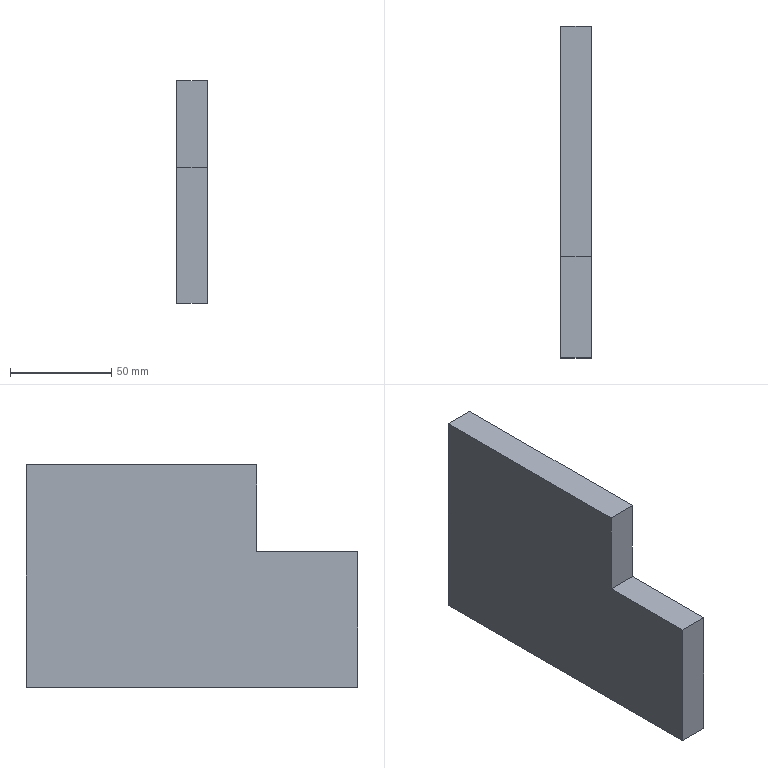Part | STEP file | Positioning_id1518_x_t | 1 solid | 8 faces | box 15 x 164 x 110 mm | volume 238350 mm3 | plane 8
STEP:
#1=CARTESIAN_POINT('',(0.,0.,0.));
#2=DIRECTION('',(0.,0.,1.));
#3=DIRECTION('',(1.,0.,0.));
#4=AXIS2_PLACEMENT_3D('',#1,#2,#3);
#5=CARTESIAN_POINT('',(-808.002,510.,100.995));
#6=VERTEX_POINT('',#5);
#7=CARTESIAN_POINT('',(-793.002,510.,100.995));
#8=VERTEX_POINT('',#7);
#9=CARTESIAN_POINT('',(-808.002,510.,100.995));
#10=DIRECTION('',(1.,0.,0.));
#11=VECTOR('',#10,1.);
#12=LINE('',#9,#11);
#13=CARTESIAN_POINT('',(-808.002,460.,100.995));
#14=DIRECTION('',(0.,0.,-1.));
#15=DIRECTION('',(-1.,0.,0.));
#16=AXIS2_PLACEMENT_3D('',#13,#14,#15);
#17=PLANE('',#16);
#18=CARTESIAN_POINT('',(0.,50.));
#19=DIRECTION('',(-1.,0.));
#20=VECTOR('',#19,1.);
#21=LINE('',#18,#20);
#22=(GEOMETRIC_REPRESENTATION_CONTEXT(2)PARAMETRIC_REPRESENTATION_CONTEXT()REPRESENTATION_CONTEXT('',''));
#23=DEFINITIONAL_REPRESENTATION('',(#21),#22);
#24=PCURVE('',#17,#23);
#25=CARTESIAN_POINT('',(-808.002,510.,133.995));
#26=DIRECTION('',(0.,-1.,0.));
#27=DIRECTION('',(-1.,0.,0.));
#28=AXIS2_PLACEMENT_3D('',#25,#26,#27);
#29=PLANE('',#28);
#30=CARTESIAN_POINT('',(0.,33.));
#31=DIRECTION('',(-1.,0.));
#32=VECTOR('',#31,1.);
#33=LINE('',#30,#32);
#34=(GEOMETRIC_REPRESENTATION_CONTEXT(2)PARAMETRIC_REPRESENTATION_CONTEXT()REPRESENTATION_CONTEXT('',''));
#35=DEFINITIONAL_REPRESENTATION('',(#33),#34);
#36=PCURVE('',#29,#35);
#37=SURFACE_CURVE('',#12,(#24,#36),.PCURVE_S1.);
#38=EDGE_CURVE('',#6,#8,#37,.T.);
#39=ORIENTED_EDGE('',*,*,#38,.F.);
#40=CARTESIAN_POINT('',(-808.002,460.,100.995));
#41=VERTEX_POINT('',#40);
#42=CARTESIAN_POINT('',(-808.002,460.,100.995));
#43=DIRECTION('',(0.,1.,0.));
#44=VECTOR('',#43,1.);
#45=LINE('',#42,#44);
#46=CARTESIAN_POINT('',(0.,0.));
#47=DIRECTION('',(0.,1.));
#48=VECTOR('',#47,1.);
#49=LINE('',#46,#48);
#50=(GEOMETRIC_REPRESENTATION_CONTEXT(2)PARAMETRIC_REPRESENTATION_CONTEXT()REPRESENTATION_CONTEXT('',''));
#51=DEFINITIONAL_REPRESENTATION('',(#49),#50);
#52=PCURVE('',#17,#51);
#53=CARTESIAN_POINT('',(-808.002,497.,63.995));
#54=DIRECTION('',(-1.,0.,0.));
#55=DIRECTION('',(0.,0.,-1.));
#56=AXIS2_PLACEMENT_3D('',#53,#54,#55);
#57=PLANE('',#56);
#58=CARTESIAN_POINT('',(-37.,37.));
#59=DIRECTION('',(0.,-1.));
#60=VECTOR('',#59,1.);
#61=LINE('',#58,#60);
#62=(GEOMETRIC_REPRESENTATION_CONTEXT(2)PARAMETRIC_REPRESENTATION_CONTEXT()REPRESENTATION_CONTEXT('',''));
#63=DEFINITIONAL_REPRESENTATION('',(#61),#62);
#64=PCURVE('',#57,#63);
#65=SURFACE_CURVE('',#45,(#52,#64),.PCURVE_S1.);
#66=EDGE_CURVE('',#41,#6,#65,.T.);
#67=ORIENTED_EDGE('',*,*,#66,.F.);
#68=CARTESIAN_POINT('',(-793.002,460.,100.995));
#69=VERTEX_POINT('',#68);
#70=CARTESIAN_POINT('',(-808.002,460.,100.995));
#71=DIRECTION('',(1.,0.,0.));
#72=VECTOR('',#71,1.);
#73=LINE('',#70,#72);
#74=CARTESIAN_POINT('',(0.,0.));
#75=DIRECTION('',(-1.,0.));
#76=VECTOR('',#75,1.);
#77=LINE('',#74,#76);
#78=(GEOMETRIC_REPRESENTATION_CONTEXT(2)PARAMETRIC_REPRESENTATION_CONTEXT()REPRESENTATION_CONTEXT('',''));
#79=DEFINITIONAL_REPRESENTATION('',(#77),#78);
#80=PCURVE('',#17,#79);
#81=CARTESIAN_POINT('',(-813.002,460.,63.995));
#82=DIRECTION('',(0.,-1.,0.));
#83=DIRECTION('',(-1.,0.,0.));
#84=AXIS2_PLACEMENT_3D('',#81,#82,#83);
#85=PLANE('',#84);
#86=CARTESIAN_POINT('',(-5.,-37.));
#87=DIRECTION('',(-1.,0.));
#88=VECTOR('',#87,1.);
#89=LINE('',#86,#88);
#90=(GEOMETRIC_REPRESENTATION_CONTEXT(2)PARAMETRIC_REPRESENTATION_CONTEXT()REPRESENTATION_CONTEXT('',''));
#91=DEFINITIONAL_REPRESENTATION('',(#89),#90);
#92=PCURVE('',#85,#91);
#93=SURFACE_CURVE('',#73,(#80,#92),.PCURVE_S1.);
#94=EDGE_CURVE('',#41,#69,#93,.T.);
#95=ORIENTED_EDGE('',*,*,#94,.T.);
#96=CARTESIAN_POINT('',(-793.002,460.,100.995));
#97=DIRECTION('',(0.,1.,0.));
#98=VECTOR('',#97,1.);
#99=LINE('',#96,#98);
#100=CARTESIAN_POINT('',(-15.,0.));
#101=DIRECTION('',(0.,1.));
#102=VECTOR('',#101,1.);
#103=LINE('',#100,#102);
#104=(GEOMETRIC_REPRESENTATION_CONTEXT(2)PARAMETRIC_REPRESENTATION_CONTEXT()REPRESENTATION_CONTEXT('',''));
#105=DEFINITIONAL_REPRESENTATION('',(#103),#104);
#106=PCURVE('',#17,#105);
#107=CARTESIAN_POINT('',(-793.002,497.,63.995));
#108=DIRECTION('',(1.,0.,0.));
#109=DIRECTION('',(0.,0.,1.));
#110=AXIS2_PLACEMENT_3D('',#107,#108,#109);
#111=PLANE('',#110);
#112=CARTESIAN_POINT('',(37.,37.));
#113=DIRECTION('',(0.,-1.));
#114=VECTOR('',#113,1.);
#115=LINE('',#112,#114);
#116=(GEOMETRIC_REPRESENTATION_CONTEXT(2)PARAMETRIC_REPRESENTATION_CONTEXT()REPRESENTATION_CONTEXT('',''));
#117=DEFINITIONAL_REPRESENTATION('',(#115),#116);
#118=PCURVE('',#111,#117);
#119=SURFACE_CURVE('',#99,(#106,#118),.PCURVE_S1.);
#120=EDGE_CURVE('',#69,#8,#119,.T.);
#121=ORIENTED_EDGE('',*,*,#120,.T.);
#122=EDGE_LOOP('',(#39,#67,#95,#121));
#123=FACE_BOUND('',#122,.T.);
#124=ADVANCED_FACE('',(#123),#17,.F.);
#125=CARTESIAN_POINT('',(-793.002,510.,143.995));
#126=VERTEX_POINT('',#125);
#127=CARTESIAN_POINT('',(-793.002,510.,100.995));
#128=DIRECTION('',(0.,0.,1.));
#129=VECTOR('',#128,1.);
#130=LINE('',#127,#129);
#131=CARTESIAN_POINT('',(-15.,33.));
#132=DIRECTION('',(0.,-1.));
#133=VECTOR('',#132,1.);
#134=LINE('',#131,#133);
#135=(GEOMETRIC_REPRESENTATION_CONTEXT(2)PARAMETRIC_REPRESENTATION_CONTEXT()REPRESENTATION_CONTEXT('',''));
#136=DEFINITIONAL_REPRESENTATION('',(#134),#135);
#137=PCURVE('',#29,#136);
#138=CARTESIAN_POINT('',(37.,-13.));
#139=DIRECTION('',(1.,0.));
#140=VECTOR('',#139,1.);
#141=LINE('',#138,#140);
#142=(GEOMETRIC_REPRESENTATION_CONTEXT(2)PARAMETRIC_REPRESENTATION_CONTEXT()REPRESENTATION_CONTEXT('',''));
#143=DEFINITIONAL_REPRESENTATION('',(#141),#142);
#144=PCURVE('',#111,#143);
#145=SURFACE_CURVE('',#130,(#137,#144),.PCURVE_S1.);
#146=EDGE_CURVE('',#8,#126,#145,.T.);
#147=ORIENTED_EDGE('',*,*,#146,.T.);
#148=CARTESIAN_POINT('',(-808.002,510.,143.995));
#149=VERTEX_POINT('',#148);
#150=CARTESIAN_POINT('',(-808.002,510.,143.995));
#151=DIRECTION('',(1.,0.,0.));
#152=VECTOR('',#151,1.);
#153=LINE('',#150,#152);
#154=CARTESIAN_POINT('',(0.,-10.));
#155=DIRECTION('',(-1.,0.));
#156=VECTOR('',#155,1.);
#157=LINE('',#154,#156);
#158=(GEOMETRIC_REPRESENTATION_CONTEXT(2)PARAMETRIC_REPRESENTATION_CONTEXT()REPRESENTATION_CONTEXT('',''));
#159=DEFINITIONAL_REPRESENTATION('',(#157),#158);
#160=PCURVE('',#29,#159);
#161=CARTESIAN_POINT('',(-813.002,497.,143.995));
#162=DIRECTION('',(0.,0.,1.));
#163=DIRECTION('',(-1.,0.,0.));
#164=AXIS2_PLACEMENT_3D('',#161,#162,#163);
#165=PLANE('',#164);
#166=CARTESIAN_POINT('',(-5.,-13.));
#167=DIRECTION('',(-1.,0.));
#168=VECTOR('',#167,1.);
#169=LINE('',#166,#168);
#170=(GEOMETRIC_REPRESENTATION_CONTEXT(2)PARAMETRIC_REPRESENTATION_CONTEXT()REPRESENTATION_CONTEXT('',''));
#171=DEFINITIONAL_REPRESENTATION('',(#169),#170);
#172=PCURVE('',#165,#171);
#173=SURFACE_CURVE('',#153,(#160,#172),.PCURVE_S1.);
#174=EDGE_CURVE('',#149,#126,#173,.T.);
#175=ORIENTED_EDGE('',*,*,#174,.F.);
#176=CARTESIAN_POINT('',(-808.002,510.,100.995));
#177=DIRECTION('',(0.,0.,1.));
#178=VECTOR('',#177,1.);
#179=LINE('',#176,#178);
#180=CARTESIAN_POINT('',(0.,33.));
#181=DIRECTION('',(0.,-1.));
#182=VECTOR('',#181,1.);
#183=LINE('',#180,#182);
#184=(GEOMETRIC_REPRESENTATION_CONTEXT(2)PARAMETRIC_REPRESENTATION_CONTEXT()REPRESENTATION_CONTEXT('',''));
#185=DEFINITIONAL_REPRESENTATION('',(#183),#184);
#186=PCURVE('',#29,#185);
#187=CARTESIAN_POINT('',(-37.,-13.));
#188=DIRECTION('',(-1.,0.));
#189=VECTOR('',#188,1.);
#190=LINE('',#187,#189);
#191=(GEOMETRIC_REPRESENTATION_CONTEXT(2)PARAMETRIC_REPRESENTATION_CONTEXT()REPRESENTATION_CONTEXT('',''));
#192=DEFINITIONAL_REPRESENTATION('',(#190),#191);
#193=PCURVE('',#57,#192);
#194=SURFACE_CURVE('',#179,(#186,#193),.PCURVE_S1.);
#195=EDGE_CURVE('',#6,#149,#194,.T.);
#196=ORIENTED_EDGE('',*,*,#195,.F.);
#197=ORIENTED_EDGE('',*,*,#38,.T.);
#198=EDGE_LOOP('',(#147,#175,#196,#197));
#199=FACE_BOUND('',#198,.T.);
#200=ADVANCED_FACE('',(#199),#29,.T.);
#201=CARTESIAN_POINT('',(-793.002,460.,33.995));
#202=VERTEX_POINT('',#201);
#203=CARTESIAN_POINT('',(-808.002,460.,33.995));
#204=VERTEX_POINT('',#203);
#205=CARTESIAN_POINT('',(-793.002,460.,33.995));
#206=DIRECTION('',(-1.,0.,0.));
#207=VECTOR('',#206,1.);
#208=LINE('',#205,#207);
#209=CARTESIAN_POINT('',(-813.002,497.,33.995));
#210=DIRECTION('',(0.,0.,-1.));
#211=DIRECTION('',(1.,0.,0.));
#212=AXIS2_PLACEMENT_3D('',#209,#210,#211);
#213=PLANE('',#212);
#214=CARTESIAN_POINT('',(20.,37.));
#215=DIRECTION('',(-1.,0.));
#216=VECTOR('',#215,1.);
#217=LINE('',#214,#216);
#218=(GEOMETRIC_REPRESENTATION_CONTEXT(2)PARAMETRIC_REPRESENTATION_CONTEXT()REPRESENTATION_CONTEXT('',''));
#219=DEFINITIONAL_REPRESENTATION('',(#217),#218);
#220=PCURVE('',#213,#219);
#221=CARTESIAN_POINT('',(-20.,30.));
#222=DIRECTION('',(1.,0.));
#223=VECTOR('',#222,1.);
#224=LINE('',#221,#223);
#225=(GEOMETRIC_REPRESENTATION_CONTEXT(2)PARAMETRIC_REPRESENTATION_CONTEXT()REPRESENTATION_CONTEXT('',''));
#226=DEFINITIONAL_REPRESENTATION('',(#224),#225);
#227=PCURVE('',#85,#226);
#228=SURFACE_CURVE('',#208,(#220,#227),.PCURVE_S1.);
#229=EDGE_CURVE('',#202,#204,#228,.T.);
#230=ORIENTED_EDGE('',*,*,#229,.T.);
#231=CARTESIAN_POINT('',(-808.002,624.,33.995));
#232=VERTEX_POINT('',#231);
#233=CARTESIAN_POINT('',(-808.002,624.,33.995));
#234=DIRECTION('',(0.,-1.,0.));
#235=VECTOR('',#234,1.);
#236=LINE('',#233,#235);
#237=CARTESIAN_POINT('',(5.,-127.));
#238=DIRECTION('',(0.,1.));
#239=VECTOR('',#238,1.);
#240=LINE('',#237,#239);
#241=(GEOMETRIC_REPRESENTATION_CONTEXT(2)PARAMETRIC_REPRESENTATION_CONTEXT()REPRESENTATION_CONTEXT('',''));
#242=DEFINITIONAL_REPRESENTATION('',(#240),#241);
#243=PCURVE('',#213,#242);
#244=CARTESIAN_POINT('',(30.,-127.));
#245=DIRECTION('',(0.,1.));
#246=VECTOR('',#245,1.);
#247=LINE('',#244,#246);
#248=(GEOMETRIC_REPRESENTATION_CONTEXT(2)PARAMETRIC_REPRESENTATION_CONTEXT()REPRESENTATION_CONTEXT('',''));
#249=DEFINITIONAL_REPRESENTATION('',(#247),#248);
#250=PCURVE('',#57,#249);
#251=SURFACE_CURVE('',#236,(#243,#250),.PCURVE_S1.);
#252=EDGE_CURVE('',#232,#204,#251,.T.);
#253=ORIENTED_EDGE('',*,*,#252,.F.);
#254=CARTESIAN_POINT('',(-793.002,624.,33.995));
#255=VERTEX_POINT('',#254);
#256=CARTESIAN_POINT('',(-808.002,624.,33.995));
#257=DIRECTION('',(1.,0.,0.));
#258=VECTOR('',#257,1.);
#259=LINE('',#256,#258);
#260=CARTESIAN_POINT('',(5.,-127.));
#261=DIRECTION('',(1.,0.));
#262=VECTOR('',#261,1.);
#263=LINE('',#260,#262);
#264=(GEOMETRIC_REPRESENTATION_CONTEXT(2)PARAMETRIC_REPRESENTATION_CONTEXT()REPRESENTATION_CONTEXT('',''));
#265=DEFINITIONAL_REPRESENTATION('',(#263),#264);
#266=PCURVE('',#213,#265);
#267=CARTESIAN_POINT('',(-813.002,624.,63.995));
#268=DIRECTION('',(0.,1.,0.));
#269=DIRECTION('',(1.,0.,0.));
#270=AXIS2_PLACEMENT_3D('',#267,#268,#269);
#271=PLANE('',#270);
#272=CARTESIAN_POINT('',(5.,30.));
#273=DIRECTION('',(1.,0.));
#274=VECTOR('',#273,1.);
#275=LINE('',#272,#274);
#276=(GEOMETRIC_REPRESENTATION_CONTEXT(2)PARAMETRIC_REPRESENTATION_CONTEXT()REPRESENTATION_CONTEXT('',''));
#277=DEFINITIONAL_REPRESENTATION('',(#275),#276);
#278=PCURVE('',#271,#277);
#279=SURFACE_CURVE('',#259,(#266,#278),.PCURVE_S1.);
#280=EDGE_CURVE('',#232,#255,#279,.T.);
#281=ORIENTED_EDGE('',*,*,#280,.T.);
#282=CARTESIAN_POINT('',(-793.002,460.,33.995));
#283=DIRECTION('',(0.,1.,0.));
#284=VECTOR('',#283,1.);
#285=LINE('',#282,#284);
#286=CARTESIAN_POINT('',(20.,37.));
#287=DIRECTION('',(0.,-1.));
#288=VECTOR('',#287,1.);
#289=LINE('',#286,#288);
#290=(GEOMETRIC_REPRESENTATION_CONTEXT(2)PARAMETRIC_REPRESENTATION_CONTEXT()REPRESENTATION_CONTEXT('',''));
#291=DEFINITIONAL_REPRESENTATION('',(#289),#290);
#292=PCURVE('',#213,#291);
#293=CARTESIAN_POINT('',(-30.,37.));
#294=DIRECTION('',(0.,-1.));
#295=VECTOR('',#294,1.);
#296=LINE('',#293,#295);
#297=(GEOMETRIC_REPRESENTATION_CONTEXT(2)PARAMETRIC_REPRESENTATION_CONTEXT()REPRESENTATION_CONTEXT('',''));
#298=DEFINITIONAL_REPRESENTATION('',(#296),#297);
#299=PCURVE('',#111,#298);
#300=SURFACE_CURVE('',#285,(#292,#299),.PCURVE_S1.);
#301=EDGE_CURVE('',#202,#255,#300,.T.);
#302=ORIENTED_EDGE('',*,*,#301,.F.);
#303=EDGE_LOOP('',(#230,#253,#281,#302));
#304=FACE_BOUND('',#303,.T.);
#305=ADVANCED_FACE('',(#304),#213,.T.);
#306=CARTESIAN_POINT('',(-793.002,460.,100.995));
#307=DIRECTION('',(0.,0.,-1.));
#308=VECTOR('',#307,1.);
#309=LINE('',#306,#308);
#310=CARTESIAN_POINT('',(-20.,-37.));
#311=DIRECTION('',(0.,1.));
#312=VECTOR('',#311,1.);
#313=LINE('',#310,#312);
#314=(GEOMETRIC_REPRESENTATION_CONTEXT(2)PARAMETRIC_REPRESENTATION_CONTEXT()REPRESENTATION_CONTEXT('',''));
#315=DEFINITIONAL_REPRESENTATION('',(#313),#314);
#316=PCURVE('',#85,#315);
#317=CARTESIAN_POINT('',(37.,37.));
#318=DIRECTION('',(-1.,0.));
#319=VECTOR('',#318,1.);
#320=LINE('',#317,#319);
#321=(GEOMETRIC_REPRESENTATION_CONTEXT(2)PARAMETRIC_REPRESENTATION_CONTEXT()REPRESENTATION_CONTEXT('',''));
#322=DEFINITIONAL_REPRESENTATION('',(#320),#321);
#323=PCURVE('',#111,#322);
#324=SURFACE_CURVE('',#309,(#316,#323),.PCURVE_S1.);
#325=EDGE_CURVE('',#69,#202,#324,.T.);
#326=ORIENTED_EDGE('',*,*,#325,.F.);
#327=ORIENTED_EDGE('',*,*,#94,.F.);
#328=CARTESIAN_POINT('',(-808.002,460.,33.995));
#329=DIRECTION('',(0.,0.,1.));
#330=VECTOR('',#329,1.);
#331=LINE('',#328,#330);
#332=CARTESIAN_POINT('',(-5.,30.));
#333=DIRECTION('',(0.,-1.));
#334=VECTOR('',#333,1.);
#335=LINE('',#332,#334);
#336=(GEOMETRIC_REPRESENTATION_CONTEXT(2)PARAMETRIC_REPRESENTATION_CONTEXT()REPRESENTATION_CONTEXT('',''));
#337=DEFINITIONAL_REPRESENTATION('',(#335),#336);
#338=PCURVE('',#85,#337);
#339=CARTESIAN_POINT('',(30.,37.));
#340=DIRECTION('',(-1.,0.));
#341=VECTOR('',#340,1.);
#342=LINE('',#339,#341);
#343=(GEOMETRIC_REPRESENTATION_CONTEXT(2)PARAMETRIC_REPRESENTATION_CONTEXT()REPRESENTATION_CONTEXT('',''));
#344=DEFINITIONAL_REPRESENTATION('',(#342),#343);
#345=PCURVE('',#57,#344);
#346=SURFACE_CURVE('',#331,(#338,#345),.PCURVE_S1.);
#347=EDGE_CURVE('',#204,#41,#346,.T.);
#348=ORIENTED_EDGE('',*,*,#347,.F.);
#349=ORIENTED_EDGE('',*,*,#229,.F.);
#350=EDGE_LOOP('',(#326,#327,#348,#349));
#351=FACE_BOUND('',#350,.T.);
#352=ADVANCED_FACE('',(#351),#85,.T.);
#353=CARTESIAN_POINT('',(-808.002,624.,143.995));
#354=VERTEX_POINT('',#353);
#355=CARTESIAN_POINT('',(-793.002,624.,143.995));
#356=VERTEX_POINT('',#355);
#357=CARTESIAN_POINT('',(-808.002,624.,143.995));
#358=DIRECTION('',(1.,0.,0.));
#359=VECTOR('',#358,1.);
#360=LINE('',#357,#359);
#361=CARTESIAN_POINT('',(5.,-80.));
#362=DIRECTION('',(1.,0.));
#363=VECTOR('',#362,1.);
#364=LINE('',#361,#363);
#365=(GEOMETRIC_REPRESENTATION_CONTEXT(2)PARAMETRIC_REPRESENTATION_CONTEXT()REPRESENTATION_CONTEXT('',''));
#366=DEFINITIONAL_REPRESENTATION('',(#364),#365);
#367=PCURVE('',#271,#366);
#368=CARTESIAN_POINT('',(-5.,-127.));
#369=DIRECTION('',(-1.,0.));
#370=VECTOR('',#369,1.);
#371=LINE('',#368,#370);
#372=(GEOMETRIC_REPRESENTATION_CONTEXT(2)PARAMETRIC_REPRESENTATION_CONTEXT()REPRESENTATION_CONTEXT('',''));
#373=DEFINITIONAL_REPRESENTATION('',(#371),#372);
#374=PCURVE('',#165,#373);
#375=SURFACE_CURVE('',#360,(#367,#374),.PCURVE_S1.);
#376=EDGE_CURVE('',#354,#356,#375,.T.);
#377=ORIENTED_EDGE('',*,*,#376,.T.);
#378=CARTESIAN_POINT('',(-793.002,624.,33.995));
#379=DIRECTION('',(0.,0.,1.));
#380=VECTOR('',#379,1.);
#381=LINE('',#378,#380);
#382=CARTESIAN_POINT('',(20.,30.));
#383=DIRECTION('',(0.,-1.));
#384=VECTOR('',#383,1.);
#385=LINE('',#382,#384);
#386=(GEOMETRIC_REPRESENTATION_CONTEXT(2)PARAMETRIC_REPRESENTATION_CONTEXT()REPRESENTATION_CONTEXT('',''));
#387=DEFINITIONAL_REPRESENTATION('',(#385),#386);
#388=PCURVE('',#271,#387);
#389=CARTESIAN_POINT('',(-30.,-127.));
#390=DIRECTION('',(1.,0.));
#391=VECTOR('',#390,1.);
#392=LINE('',#389,#391);
#393=(GEOMETRIC_REPRESENTATION_CONTEXT(2)PARAMETRIC_REPRESENTATION_CONTEXT()REPRESENTATION_CONTEXT('',''));
#394=DEFINITIONAL_REPRESENTATION('',(#392),#393);
#395=PCURVE('',#111,#394);
#396=SURFACE_CURVE('',#381,(#388,#395),.PCURVE_S1.);
#397=EDGE_CURVE('',#255,#356,#396,.T.);
#398=ORIENTED_EDGE('',*,*,#397,.F.);
#399=ORIENTED_EDGE('',*,*,#280,.F.);
#400=CARTESIAN_POINT('',(-808.002,624.,143.995));
#401=DIRECTION('',(0.,0.,-1.));
#402=VECTOR('',#401,1.);
#403=LINE('',#400,#402);
#404=CARTESIAN_POINT('',(5.,-80.));
#405=DIRECTION('',(0.,1.));
#406=VECTOR('',#405,1.);
#407=LINE('',#404,#406);
#408=(GEOMETRIC_REPRESENTATION_CONTEXT(2)PARAMETRIC_REPRESENTATION_CONTEXT()REPRESENTATION_CONTEXT('',''));
#409=DEFINITIONAL_REPRESENTATION('',(#407),#408);
#410=PCURVE('',#271,#409);
#411=CARTESIAN_POINT('',(-80.,-127.));
#412=DIRECTION('',(1.,0.));
#413=VECTOR('',#412,1.);
#414=LINE('',#411,#413);
#415=(GEOMETRIC_REPRESENTATION_CONTEXT(2)PARAMETRIC_REPRESENTATION_CONTEXT()REPRESENTATION_CONTEXT('',''));
#416=DEFINITIONAL_REPRESENTATION('',(#414),#415);
#417=PCURVE('',#57,#416);
#418=SURFACE_CURVE('',#403,(#410,#417),.PCURVE_S1.);
#419=EDGE_CURVE('',#354,#232,#418,.T.);
#420=ORIENTED_EDGE('',*,*,#419,.F.);
#421=EDGE_LOOP('',(#377,#398,#399,#420));
#422=FACE_BOUND('',#421,.T.);
#423=ADVANCED_FACE('',(#422),#271,.T.);
#424=CARTESIAN_POINT('',(-808.002,510.,143.995));
#425=DIRECTION('',(0.,1.,0.));
#426=VECTOR('',#425,1.);
#427=LINE('',#424,#426);
#428=CARTESIAN_POINT('',(-80.,-13.));
#429=DIRECTION('',(0.,-1.));
#430=VECTOR('',#429,1.);
#431=LINE('',#428,#430);
#432=(GEOMETRIC_REPRESENTATION_CONTEXT(2)PARAMETRIC_REPRESENTATION_CONTEXT()REPRESENTATION_CONTEXT('',''));
#433=DEFINITIONAL_REPRESENTATION('',(#431),#432);
#434=PCURVE('',#57,#433);
#435=CARTESIAN_POINT('',(-5.,-13.));
#436=DIRECTION('',(0.,-1.));
#437=VECTOR('',#436,1.);
#438=LINE('',#435,#437);
#439=(GEOMETRIC_REPRESENTATION_CONTEXT(2)PARAMETRIC_REPRESENTATION_CONTEXT()REPRESENTATION_CONTEXT('',''));
#440=DEFINITIONAL_REPRESENTATION('',(#438),#439);
#441=PCURVE('',#165,#440);
#442=SURFACE_CURVE('',#427,(#434,#441),.PCURVE_S1.);
#443=EDGE_CURVE('',#149,#354,#442,.T.);
#444=ORIENTED_EDGE('',*,*,#443,.T.);
#445=ORIENTED_EDGE('',*,*,#419,.T.);
#446=ORIENTED_EDGE('',*,*,#252,.T.);
#447=ORIENTED_EDGE('',*,*,#347,.T.);
#448=ORIENTED_EDGE('',*,*,#66,.T.);
#449=ORIENTED_EDGE('',*,*,#195,.T.);
#450=EDGE_LOOP('',(#444,#445,#446,#447,#448,#449));
#451=FACE_BOUND('',#450,.T.);
#452=ADVANCED_FACE('',(#451),#57,.T.);
#453=CARTESIAN_POINT('',(-793.002,624.,143.995));
#454=DIRECTION('',(0.,-1.,0.));
#455=VECTOR('',#454,1.);
#456=LINE('',#453,#455);
#457=CARTESIAN_POINT('',(-20.,-127.));
#458=DIRECTION('',(0.,1.));
#459=VECTOR('',#458,1.);
#460=LINE('',#457,#459);
#461=(GEOMETRIC_REPRESENTATION_CONTEXT(2)PARAMETRIC_REPRESENTATION_CONTEXT()REPRESENTATION_CONTEXT('',''));
#462=DEFINITIONAL_REPRESENTATION('',(#460),#461);
#463=PCURVE('',#165,#462);
#464=CARTESIAN_POINT('',(80.,-127.));
#465=DIRECTION('',(0.,1.));
#466=VECTOR('',#465,1.);
#467=LINE('',#464,#466);
#468=(GEOMETRIC_REPRESENTATION_CONTEXT(2)PARAMETRIC_REPRESENTATION_CONTEXT()REPRESENTATION_CONTEXT('',''));
#469=DEFINITIONAL_REPRESENTATION('',(#467),#468);
#470=PCURVE('',#111,#469);
#471=SURFACE_CURVE('',#456,(#463,#470),.PCURVE_S1.);
#472=EDGE_CURVE('',#356,#126,#471,.T.);
#473=ORIENTED_EDGE('',*,*,#472,.F.);
#474=ORIENTED_EDGE('',*,*,#376,.F.);
#475=ORIENTED_EDGE('',*,*,#443,.F.);
#476=ORIENTED_EDGE('',*,*,#174,.T.);
#477=EDGE_LOOP('',(#473,#474,#475,#476));
#478=FACE_BOUND('',#477,.T.);
#479=ADVANCED_FACE('',(#478),#165,.T.);
#480=ORIENTED_EDGE('',*,*,#120,.F.);
#481=ORIENTED_EDGE('',*,*,#325,.T.);
#482=ORIENTED_EDGE('',*,*,#301,.T.);
#483=ORIENTED_EDGE('',*,*,#397,.T.);
#484=ORIENTED_EDGE('',*,*,#472,.T.);
#485=ORIENTED_EDGE('',*,*,#146,.F.);
#486=EDGE_LOOP('',(#480,#481,#482,#483,#484,#485));
#487=FACE_BOUND('',#486,.T.);
#488=ADVANCED_FACE('',(#487),#111,.T.);
#489=CLOSED_SHELL('',(#124,#200,#305,#352,#423,#452,#479,#488));
#490=MANIFOLD_SOLID_BREP('',#489);
#491=(LENGTH_UNIT()NAMED_UNIT(*)SI_UNIT(.MILLI.,.METRE.));
#492=UNCERTAINTY_MEASURE_WITH_UNIT(LENGTH_MEASURE(0.0000001),#491,'','');
#493=(NAMED_UNIT(*)PLANE_ANGLE_UNIT()SI_UNIT($,.RADIAN.));
#494=(NAMED_UNIT(*)SI_UNIT($,.STERADIAN.)SOLID_ANGLE_UNIT());
#495=(GEOMETRIC_REPRESENTATION_CONTEXT(3)GLOBAL_UNCERTAINTY_ASSIGNED_CONTEXT((#492))GLOBAL_UNIT_ASSIGNED_CONTEXT((#491,#493,#494))REPRESENTATION_CONTEXT('',''));
#496=ADVANCED_BREP_SHAPE_REPRESENTATION('',(#4,#490),#495);